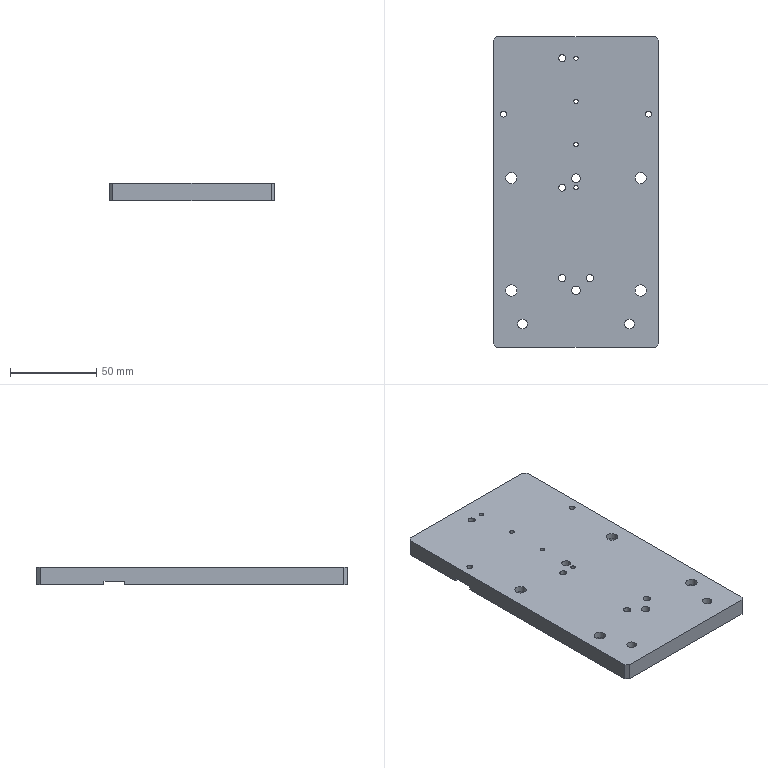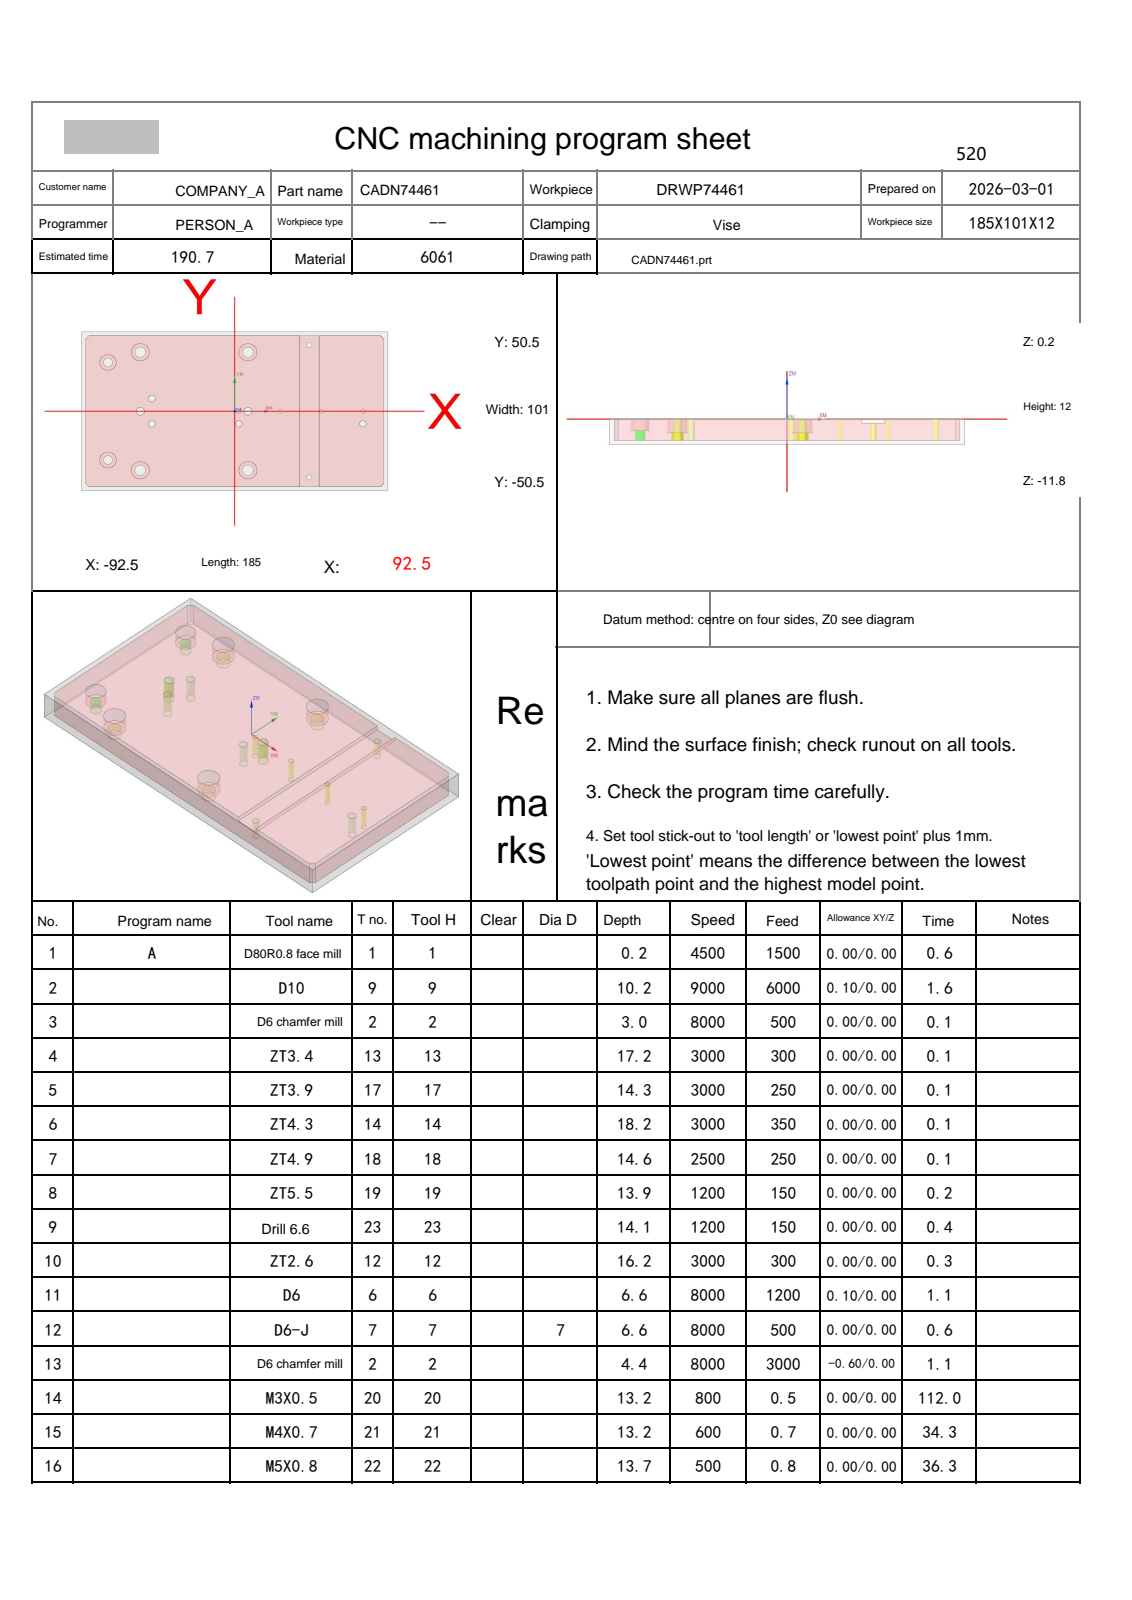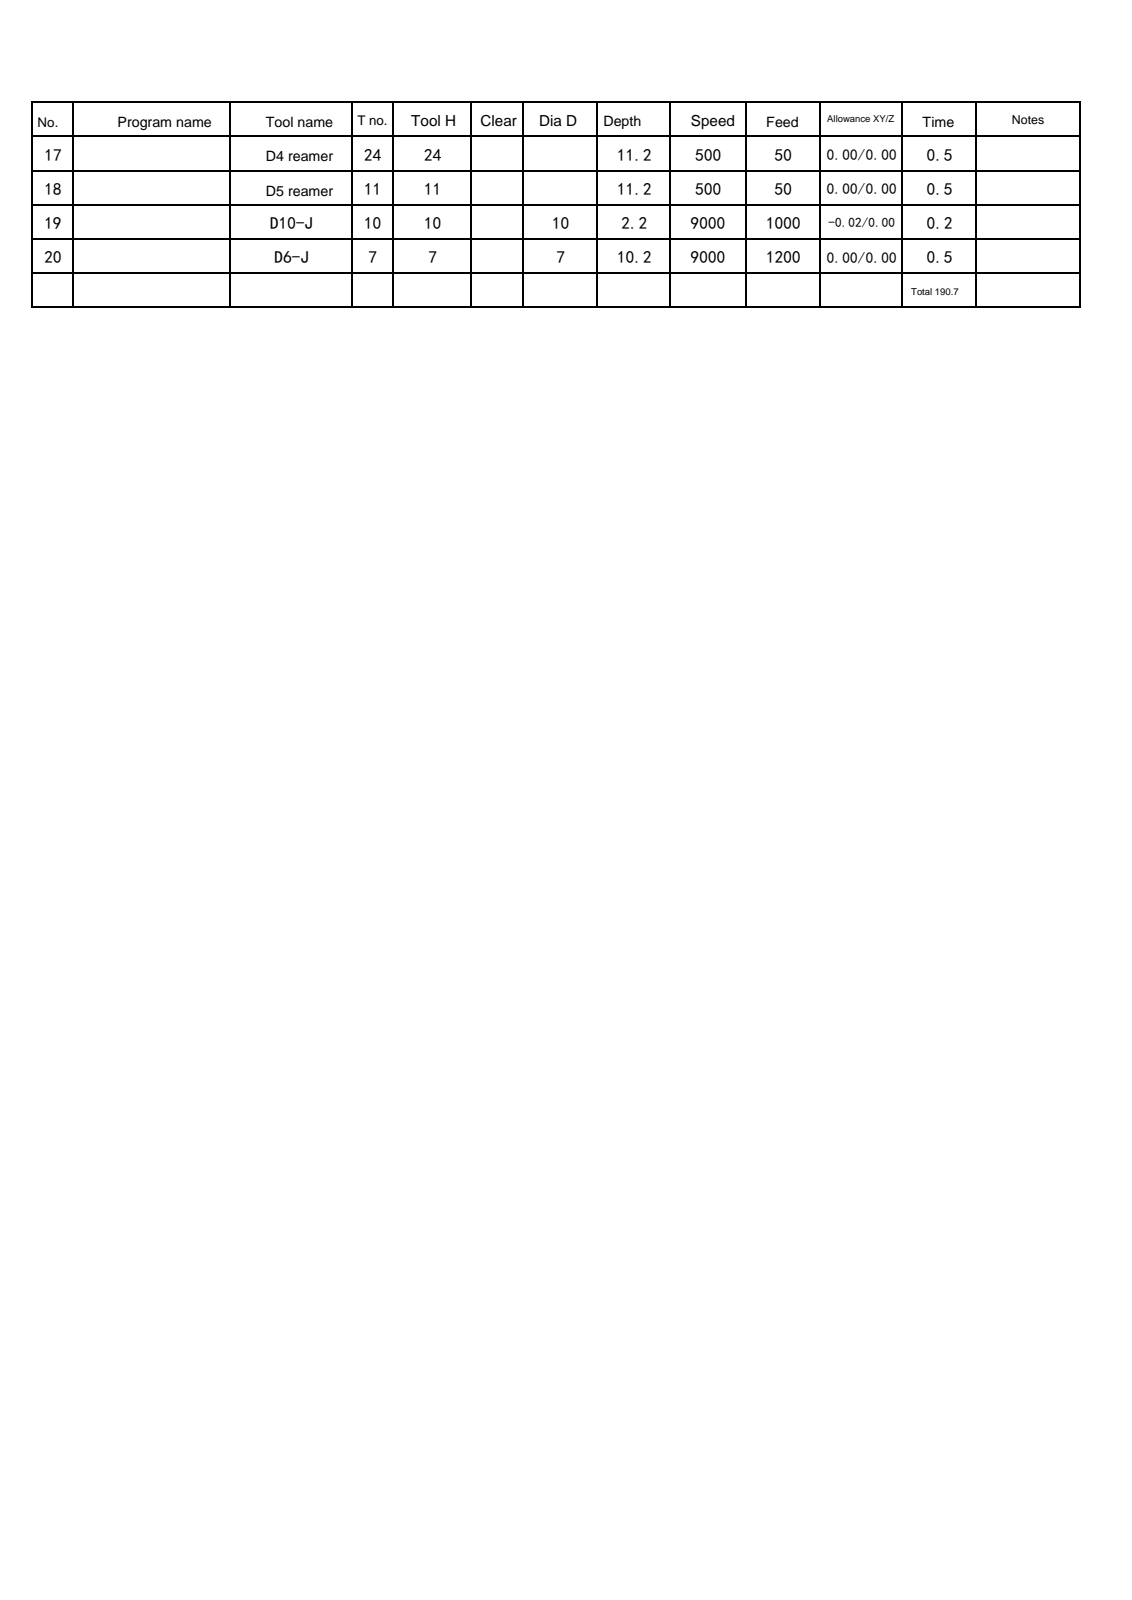NC program | NX | posted by the shop | part box 96 x 180 x 10 mm
Whole program:
%
O0001
(Machine time: 363.87 MIN)
(===Total Tool:18===)
(T1=D80R0.8 face mill D=80.  R=0.8  D-  H01 Z=0.    )
(T9=D10     D=10.  R=0.   D-  H09 Z=-10.  )
(T2=D6 chamfer mill   D=6.   R=0.   D-  H02 Z=-4.2  )
(T13=ZT3.4  D=3.4  DR_a=118 D-  H13 Z=-17.  )
(T17=ZT3.9  D=3.9  DR_a=120 D-  H17 Z=-14.13)
(T14=ZT4.3  D=4.3  DR_a=118 D-  H14 Z=-18.  )
(T18=ZT4.9  D=4.9  DR_a=120 D-  H18 Z=-14.41)
(T19=ZT5.5  D=5.5  DR_a=118 D-  H19 Z=-13.65)
(T23=drill 6.6  D=6.6  DR_a=120 D-  H23 Z=-13.91)
(T12=ZT2.6  D=2.6  DR_a=118 D-  H12 Z=-16.  )
(T6=D6      D=6.   R=0.   D-  H06 Z=-6.4  )
(T7=D6-J    D=6.   R=0.   D7  H07 Z=-10.  )
(T20=M3X0.5 D=2.5  DR_a=180 D-  H20 Z=-13.  )
(T21=M4X0.7 D=3.3  DR_a=180 D-  H21 Z=-13.  )
(T22=M5X0.8 D=4.2  DR_a=180 D-  H22 Z=-13.5 )
(T24=D4 reamer   D=4.   DR_a=180 D-  H24 Z=-11.  )
(T11=D5 reamer   D=5.   DR_a=180 D-  H11 Z=-11.  )
(T10=D10-J  D=10.  R=0.   D10 H10 Z=-2.   )
G80 G90 G17 G49 G40
G91 G28 Z0
M01
N1 T01 M06
(D80R0.8 face mill  D=80. R=0.8 H=01 ce=0.00 di=0.00)
G00 G90 G54 X-135. Y44. M03 S4500
G43 H01 Z50.
M08
Z2.
G01 Z0.0 F1500.
X-130.
X130.
Y0.0
X-130.
Y-44.
X130.
X135.
Z2.
G00 Z50.
G91 G28 Z0.0
M05
M09
G91 G28 Z0.0
M01
N2 T09 M06
(D10  D=10. R=0. H=09 ce=0.10 di=0.00)
G00 G90 G54 X0.0 Y-53.1 M03 S8000
G43 H09 Z50.
M08
Z.5
G01 X-88. Z.386 F6000.
G02 X-91.606 Y-51.606 Z.381 I0.0 J5.1
G01 X-93.606 Y-49.606 Z.377
G02 X-95.1 Y-46. Z.372 I3.606 J3.606
G01 Y46. Z.253
G02 X-93.606 Y49.606 Z.248 I5.1 J0.0
G01 X-91.606 Y51.606 Z.244
G02 X-88. Y53.1 Z.239 I3.606 J-3.606
G01 X88. Z.011
G02 X91.606 Y51.606 Z.006 I0.0 J-5.1
G01 X93.606 Y49.606 Z.002
G02 X95.1 Y46. Z-.003 I-3.606 J-3.606
G01 Y-46. Z-.122
G02 X93.606 Y-49.606 Z-.127 I-5.1 J0.0
G01 X91.606 Y-51.606 Z-.131
G02 X88. Y-53.1 Z-.136 I-3.606 J3.606
G01 X-88. Z-.364
G02 X-91.606 Y-51.606 Z-.369 I0.0 J5.1
G01 X-93.606 Y-49.606 Z-.373
G02 X-95.1 Y-46. Z-.378 I3.606 J3.606
G01 Y46. Z-.497
G02 X-93.606 Y49.606 Z-.502 I5.1 J0.0
G01 X-91.606 Y51.606 Z-.506
G02 X-88. Y53.1 Z-.511 I3.606 J-3.606
G01 X88. Z-.739
G02 X91.606 Y51.606 Z-.744 I0.0 J-5.1
G01 X93.606 Y49.606 Z-.748
G02 X95.1 Y46. Z-.753 I-3.606 J-3.606
G01 Y-46. Z-.872
G02 X93.606 Y-49.606 Z-.877 I-5.1 J0.0
G01 X91.606 Y-51.606 Z-.881
G02 X88. Y-53.1 Z-.886 I-3.606 J3.606
G01 X-88. Z-1.114
G02 X-91.606 Y-51.606 Z-1.119 I0.0 J5.1
G01 X-93.606 Y-49.606 Z-1.123
G02 X-95.1 Y-46. Z-1.128 I3.606 J3.606
G01 Y46. Z-1.247
G02 X-93.606 Y49.606 Z-1.252 I5.1 J0.0
G01 X-91.606 Y51.606 Z-1.256
G02 X-88. Y53.1 Z-1.261 I3.606 J-3.606
G01 X88. Z-1.489
G02 X91.606 Y51.606 Z-1.494 I0.0 J-5.1
G01 X93.606 Y49.606 Z-1.498
G02 X95.1 Y46. Z-1.503 I-3.606 J-3.606
G01 Y-46. Z-1.622
G02 X93.606 Y-49.606 Z-1.627 I-5.1 J0.0
G01 X91.606 Y-51.606 Z-1.631
G02 X88. Y-53.1 Z-1.636 I-3.606 J3.606
G01 X-88. Z-1.864
G02 X-91.606 Y-51.606 Z-1.869 I0.0 J5.1
G01 X-93.606 Y-49.606 Z-1.873
G02 X-95.1 Y-46. Z-1.878 I3.606 J3.606
G01 Y46. Z-1.997
G02 X-93.606 Y49.606 Z-2.002 I5.1 J0.0
G01 X-91.606 Y51.606 Z-2.006
G02 X-88. Y53.1 Z-2.011 I3.606 J-3.606
G01 X88. Z-2.239
G02 X91.606 Y51.606 Z-2.244 I0.0 J-5.1
G01 X93.606 Y49.606 Z-2.248
G02 X95.1 Y46. Z-2.253 I-3.606 J-3.606
G01 Y-46. Z-2.372
G02 X93.606 Y-49.606 Z-2.377 I-5.1 J0.0
G01 X91.606 Y-51.606 Z-2.381
G02 X88. Y-53.1 Z-2.386 I-3.606 J3.606
G01 X-88. Z-2.614
G02 X-91.606 Y-51.606 Z-2.619 I0.0 J5.1
G01 X-93.606 Y-49.606 Z-2.623
G02 X-95.1 Y-46. Z-2.628 I3.606 J3.606
G01 Y46. Z-2.747
G02 X-93.606 Y49.606 Z-2.752 I5.1 J0.0
G01 X-91.606 Y51.606 Z-2.756
G02 X-88. Y53.1 Z-2.761 I3.606 J-3.606
G01 X88. Z-2.989
G02 X91.606 Y51.606 Z-2.994 I0.0 J-5.1
G01 X93.606 Y49.606 Z-2.998
G02 X95.1 Y46. Z-3.003 I-3.606 J-3.606
G01 Y-46. Z-3.122
G02 X93.606 Y-49.606 Z-3.127 I-5.1 J0.0
G01 X91.606 Y-51.606 Z-3.131
G02 X88. Y-53.1 Z-3.136 I-3.606 J3.606
G01 X-88. Z-3.364
G02 X-91.606 Y-51.606 Z-3.369 I0.0 J5.1
G01 X-93.606 Y-49.606 Z-3.373
G02 X-95.1 Y-46. Z-3.378 I3.606 J3.606
G01 Y46. Z-3.497
G02 X-93.606 Y49.606 Z-3.502 I5.1 J0.0
G01 X-91.606 Y51.606 Z-3.506
G02 X-88. Y53.1 Z-3.511 I3.606 J-3.606
G01 X88. Z-3.739
G02 X91.606 Y51.606 Z-3.744 I0.0 J-5.1
G01 X93.606 Y49.606 Z-3.748
G02 X95.1 Y46. Z-3.753 I-3.606 J-3.606
G01 Y-46. Z-3.872
G02 X93.606 Y-49.606 Z-3.877 I-5.1 J0.0
G01 X91.606 Y-51.606 Z-3.881
G02 X88. Y-53.1 Z-3.886 I-3.606 J3.606
G01 X-88. Z-4.114
G02 X-91.606 Y-51.606 Z-4.119 I0.0 J5.1
G01 X-93.606 Y-49.606 Z-4.123
G02 X-95.1 Y-46. Z-4.128 I3.606 J3.606
G01 Y46. Z-4.247
G02 X-93.606 Y49.606 Z-4.252 I5.1 J0.0
G01 X-91.606 Y51.606 Z-4.256
G02 X-88. Y53.1 Z-4.261 I3.606 J-3.606
G01 X88. Z-4.489
G02 X91.606 Y51.606 Z-4.494 I0.0 J-5.1
G01 X93.606 Y49.606 Z-4.498
G02 X95.1 Y46. Z-4.503 I-3.606 J-3.606
G01 Y-46. Z-4.622
G02 X93.606 Y-49.606 Z-4.627 I-5.1 J0.0
G01 X91.606 Y-51.606 Z-4.631
G02 X88. Y-53.1 Z-4.636 I-3.606 J3.606
G01 X-88. Z-4.864
G02 X-91.606 Y-51.606 Z-4.869 I0.0 J5.1
G01 X-93.606 Y-49.606 Z-4.873
G02 X-95.1 Y-46. Z-4.878 I3.606 J3.606
G01 Y46. Z-4.997
G02 X-93.606 Y49.606 Z-5.002 I5.1 J0.0
G01 X-91.606 Y51.606 Z-5.006
G02 X-88. Y53.1 Z-5.011 I3.606 J-3.606
G01 X88. Z-5.239
G02 X91.606 Y51.606 Z-5.244 I0.0 J-5.1
G01 X93.606 Y49.606 Z-5.248
G02 X95.1 Y46. Z-5.253 I-3.606 J-3.606
G01 Y-46. Z-5.372
G02 X93.606 Y-49.606 Z-5.377 I-5.1 J0.0
G01 X91.606 Y-51.606 Z-5.381
G02 X88. Y-53.1 Z-5.386 I-3.606 J3.606
G01 X-88. Z-5.614
G02 X-91.606 Y-51.606 Z-5.619 I0.0 J5.1
G01 X-93.606 Y-49.606 Z-5.623
G02 X-95.1 Y-46. Z-5.628 I3.606 J3.606
G01 Y46. Z-5.747
G02 X-93.606 Y49.606 Z-5.752 I5.1 J0.0
G01 X-91.606 Y51.606 Z-5.756
G02 X-88. Y53.1 Z-5.761 I3.606 J-3.606
G01 X88. Z-5.989
G02 X91.606 Y51.606 Z-5.994 I0.0 J-5.1
G01 X93.606 Y49.606 Z-5.998
G02 X95.1 Y46. Z-6.003 I-3.606 J-3.606
G01 Y-46. Z-6.122
G02 X93.606 Y-49.606 Z-6.127 I-5.1 J0.0
G01 X91.606 Y-51.606 Z-6.131
G02 X88. Y-53.1 Z-6.136 I-3.606 J3.606
G01 X-88. Z-6.364
G02 X-91.606 Y-51.606 Z-6.369 I0.0 J5.1
G01 X-93.606 Y-49.606 Z-6.373
G02 X-95.1 Y-46. Z-6.378 I3.606 J3.606
G01 Y46. Z-6.497
G02 X-93.606 Y49.606 Z-6.502 I5.1 J0.0
G01 X-91.606 Y51.606 Z-6.506
G02 X-88. Y53.1 Z-6.511 I3.606 J-3.606
G01 X88. Z-6.739
G02 X91.606 Y51.606 Z-6.744 I0.0 J-5.1
G01 X93.606 Y49.606 Z-6.748
G02 X95.1 Y46. Z-6.753 I-3.606 J-3.606
G01 Y-46. Z-6.872
G02 X93.606 Y-49.606 Z-6.877 I-5.1 J0.0
G01 X91.606 Y-51.606 Z-6.881
G02 X88. Y-53.1 Z-6.886 I-3.606 J3.606
G01 X-88. Z-7.114
G02 X-91.606 Y-51.606 Z-7.119 I0.0 J5.1
G01 X-93.606 Y-49.606 Z-7.123
G02 X-95.1 Y-46. Z-7.128 I3.606 J3.606
G01 Y46. Z-7.247
G02 X-93.606 Y49.606 Z-7.252 I5.1 J0.0
G01 X-91.606 Y51.606 Z-7.256
G02 X-88. Y53.1 Z-7.261 I3.606 J-3.606
G01 X88. Z-7.489
G02 X91.606 Y51.606 Z-7.494 I0.0 J-5.1
G01 X93.606 Y49.606 Z-7.498
G02 X95.1 Y46. Z-7.503 I-3.606 J-3.606
G01 Y-46. Z-7.622
G02 X93.606 Y-49.606 Z-7.627 I-5.1 J0.0
G01 X91.606 Y-51.606 Z-7.631
G02 X88. Y-53.1 Z-7.636 I-3.606 J3.606
G01 X-88. Z-7.864
G02 X-91.606 Y-51.606 Z-7.869 I0.0 J5.1
G01 X-93.606 Y-49.606 Z-7.873
G02 X-95.1 Y-46. Z-7.878 I3.606 J3.606
G01 Y46. Z-7.997
G02 X-93.606 Y49.606 Z-8.002 I5.1 J0.0
G01 X-91.606 Y51.606 Z-8.006
G02 X-88. Y53.1 Z-8.011 I3.606 J-3.606
G01 X88. Z-8.239
G02 X91.606 Y51.606 Z-8.244 I0.0 J-5.1
G01 X93.606 Y49.606 Z-8.248
G02 X95.1 Y46. Z-8.253 I-3.606 J-3.606
G01 Y-46. Z-8.372
G02 X93.606 Y-49.606 Z-8.377 I-5.1 J0.0
G01 X91.606 Y-51.606 Z-8.381
G02 X88. Y-53.1 Z-8.386 I-3.606 J3.606
G01 X-88. Z-8.614
G02 X-91.606 Y-51.606 Z-8.619 I0.0 J5.1
G01 X-93.606 Y-49.606 Z-8.623
G02 X-95.1 Y-46. Z-8.628 I3.606 J3.606
G01 Y46. Z-8.747
G02 X-93.606 Y49.606 Z-8.752 I5.1 J0.0
G01 X-91.606 Y51.606 Z-8.756
G02 X-88. Y53.1 Z-8.761 I3.606 J-3.606
G01 X88. Z-8.989
G02 X91.606 Y51.606 Z-8.994 I0.0 J-5.1
G01 X93.606 Y49.606 Z-8.998
G02 X95.1 Y46. Z-9.003 I-3.606 J-3.606
G01 Y-46. Z-9.122
G02 X93.606 Y-49.606 Z-9.127 I-5.1 J0.0
G01 X91.606 Y-51.606 Z-9.131
G02 X88. Y-53.1 Z-9.136 I-3.606 J3.606
G01 X-88. Z-9.364
G02 X-91.606 Y-51.606 Z-9.369 I0.0 J5.1
G01 X-93.606 Y-49.606 Z-9.373
G02 X-95.1 Y-46. Z-9.378 I3.606 J3.606
G01 Y46. Z-9.497
G02 X-93.606 Y49.606 Z-9.502 I5.1 J0.0
G01 X-91.606 Y51.606 Z-9.506
G02 X-88. Y53.1 Z-9.511 I3.606 J-3.606
G01 X88. Z-9.739
G02 X91.606 Y51.606 Z-9.744 I0.0 J-5.1
G01 X93.606 Y49.606 Z-9.748
G02 X95.1 Y46. Z-9.753 I-3.606 J-3.606
G01 Y-46. Z-9.872
G02 X93.606 Y-49.606 Z-9.877 I-5.1 J0.0
G01 X91.606 Y-51.606 Z-9.881
G02 X88. Y-53.1 Z-9.886 I-3.606 J3.606
G01 X0.0 Z-10.
X-88.
G02 X-91.606 Y-51.606 I0.0 J5.1
G01 X-93.606 Y-49.606
G02 X-95.1 Y-46. I3.606 J3.606
G01 Y46.
G02 X-93.606 Y49.606 I5.1 J0.0
G01 X-91.606 Y51.606
G02 X-88. Y53.1 I3.606 J-3.606
G01 X88.
G02 X91.606 Y51.606 I0.0 J-5.1
G01 X93.606 Y49.606
G02 X95.1 Y46. I-3.606 J-3.606
G01 Y-46.
G02 X93.606 Y-49.606 I-5.1 J0.0
G01 X91.606 Y-51.606
G02 X88. Y-53.1 I-3.606 J3.606
G01 X0.0
X-.5
Z-9.
G00 Z50.
G00 G90 X45. Y56.1 M03 S9000
Z50.
Z.025
G01 Z-.475 F6000.
Y49.
X44.1
Y-49.
X45.9
Y49.
X45.
X44.5
Z.025
G00 Z50.
X45. Y56.1
Z-.45
G01 Z-.95
Y49.
X44.1
Y-49.
X45.9
Y49.
X45.
X44.5
Z-.45
G00 Z.025
X45. Y56.1
Z-.925
G01 Z-1.425
Y49.
X44.1
Y-49.
X45.9
Y49.
X45.
X44.5
Z-.925
G00 Z-.45
X45. Y56.1
Z-1.4
G01 Z-1.9
Y49.
X44.1
Y-49.
X45.9
Y49.
X45.
X44.5
Z-1.4
G00 Z50.
G91 G28 Z0.0
M05
M09
G91 G28 Z0.0
M01
N3 T02 M06
(D6 chamfer mill  D=6. R=0. H=02 ce=0.00 di=0.10)
G00 G90 G54 X-76.5 Y31. M03 S8000
G43 H02 Z50.
M08
G98 G81 X-76.5 Y31. Z-.8 R1. F500.
X-57. Y37.5
X-50. Y8.
X-57. Y0.0
X-50. Y-8.
X-76.5 Y-31.
X-57. Y-37.5
X8.
X45. Y-42. Z-2.8 R-1.
X77.5 Y-8. Z-.8 R1.
Y0.0
X52.5
X27.5
X8.
X2.5 Y-8.
Y0.0
X8. Y37.5
X45. Y42. Z-2.8 R-1.
G80
G00 Z50.
G91 G28 Z0.0
M05
M09
G91 G28 Z0.0
M01
N4 T13 M06
(ZT3.4 D=3.4 DR_a=118 H=13)
G00 G90 G54 X45. Y-42. M03 S3000
G43 H13 Z50.
M08
G98 G83 X45. Y-42. Z-17. R-1. F300. Q2.
Y42.
G80
G00 Z50.
G91 G28 Z0.0
M05
M09
G91 G28 Z0.0
M01
N5 T17 M06
(ZT3.9 D=3.9 DR_a=120 H=17)
G00 G90 G54 X2.5 Y-8. M03 S3000
G43 H17 Z50.
M08
G98 G83 X2.5 Y-8. Z-14.126 R1. F250. Q2.
X77.5
G80
G00 Z50.
G91 G28 Z0.0
M05
M09
G91 G28 Z0.0
M01
N6 T14 M06
(ZT4.3 D=4.3 DR_a=118 H=14)
G00 G90 G54 X-50. Y8. M03 S3000
G43 H14 Z50.
M08
G98 G83 X-50. Y8. Z-18. R1. F350. Q3.
Y-8.
G80
G00 Z50.
G91 G28 Z0.0
M05
M09
G91 G28 Z0.0
M01
N7 T18 M06
(ZT4.9 D=4.9 DR_a=120 H=18)
G00 G90 G54 X8. Y0.0 M03 S2500
G43 H18 Z50.
M08
G98 G83 X8. Y0.0 Z-14.415 R1. F250. Q2.
X-57.
G80
G00 Z50.
G91 G28 Z0.0
M05
M09
G91 G28 Z0.0
M01
N8 T19 M06
(ZT5.5 D=5.5 DR_a=118 H=19)
G00 G90 G54 X-76.5 Y31. M03 S1200
G43 H19 Z50.
M08
G98 G83 X-76.5 Y31. Z-13.652 R1. F150. Q2.
Y-31.
G80
G00 Z50.
G91 G28 Z0.0
M05
M09
G91 G28 Z0.0
M01
N9 T23 M06
(drill 6.6 D=6.6 DR_a=120 H=23)
G00 G90 G54 X-57. Y-37.5 M03 S1200
G43 H23 Z50.
M08
G98 G83 X-57. Y-37.5 Z-13.905 R1. F150. Q2.
X8.
Y37.5
X-57.
G80
G00 Z50.
G91 G28 Z0.0
M05
M09
G91 G28 Z0.0
M01
N10 T12 M06
(ZT2.6 D=2.6 DR_a=118 H=12)
G00 G90 G54 X2.5 Y0.0 M03 S3000
G43 H12 Z50.
M08
G98 G83 X2.5 Y0.0 Z-16. R1. F300. Q2.
X27.5
X52.5
X77.5
G80
G00 Z50.
G91 G28 Z0.0
M05
M09
G91 G28 Z0.0
M01
N11 T06 M06
(D6  D=6. R=0. H=06 ce=0.10 di=0.00)
G00 G90 G54 X-76.5 Y31. M03 S8000
G43 H06 Z50.
M08
Z.5
G03 X-75.55 Y31.95 I0.0 J.95 F1200.
X-76.5 Y32.9 I-.95 J0.0
X-76.5 Y32.9 Z0.0 I0.0 J-1.9
X-76.5 Y32.9 Z-.5 I0.0 J-1.9
X-76.5 Y32.9 Z-1. I0.0 J-1.9
X-76.5 Y32.9 Z-1.5 I0.0 J-1.9
X-76.5 Y32.9 Z-2. I0.0 J-1.9
X-76.5 Y32.9 Z-2.5 I0.0 J-1.9
X-76.5 Y32.9 Z-3. I0.0 J-1.9
X-76.5 Y32.9 Z-3.5 I0.0 J-1.9
X-76.5 Y32.9 Z-4. I0.0 J-1.9
X-76.5 Y32.9 Z-4.5 I0.0 J-1.9
X-76.5 Y32.9 Z-5. I0.0 J-1.9
X-74.693 Y31.587 Z-5.4 I0.0 J-1.9
X-76.5 Y32.9 I-1.807 J-.587
X-78.4 Y31. I0.0 J-1.9
X-76.5 Y29.1 I1.9 J0.0
X-74.6 Y31. I0.0 J1.9
X-74.693 Y31.587 I-1.9 J0.0
X-75.596 Y32.244 I-.904 J-.294
X-76.546 Y31.294 I0.0 J-.95
X-76.5 Y31. I.95 J0.0
G00 Z50.
Y-31.
Z.5
G03 X-75.55 Y-30.05 I0.0 J.95
X-76.5 Y-29.1 I-.95 J0.0
X-76.5 Y-29.1 Z0.0 I0.0 J-1.9
X-76.5 Y-29.1 Z-.5 I0.0 J-1.9
X-76.5 Y-29.1 Z-1. I0.0 J-1.9
X-76.5 Y-29.1 Z-1.5 I0.0 J-1.9
X-76.5 Y-29.1 Z-2. I0.0 J-1.9
X-76.5 Y-29.1 Z-2.5 I0.0 J-1.9
X-76.5 Y-29.1 Z-3. I0.0 J-1.9
X-76.5 Y-29.1 Z-3.5 I0.0 J-1.9
X-76.5 Y-29.1 Z-4. I0.0 J-1.9
X-76.5 Y-29.1 Z-4.5 I0.0 J-1.9
X-76.5 Y-29.1 Z-5. I0.0 J-1.9
X-74.693 Y-30.413 Z-5.4 I0.0 J-1.9
X-76.5 Y-29.1 I-1.807 J-.587
X-78.4 Y-31. I0.0 J-1.9
X-76.5 Y-32.9 I1.9 J0.0
X-74.6 Y-31. I0.0 J1.9
X-74.693 Y-30.413 I-1.9 J0.0
X-75.596 Y-29.756 I-.904 J-.294
X-76.546 Y-30.706 I0.0 J-.95
X-76.5 Y-31. I.95 J0.0
G00 Z50.
G00 G90 X-57. Y-37.5 M03 S8000
Z50.
Z.5
G03 X-55.8 Y-36.3 I0.0 J1.2 F1200.
X-57. Y-35.1 I-1.2 J0.0
X-57. Y-35.1 Z0.0 I0.0 J-2.4
X-57. Y-35.1 Z-.5 I0.0 J-2.4
X-57. Y-35.1 Z-1. I0.0 J-2.4
X-57. Y-35.1 Z-1.5 I0.0 J-2.4
X-57. Y-35.1 Z-2. I0.0 J-2.4
X-57. Y-35.1 Z-2.5 I0.0 J-2.4
X-57. Y-35.1 Z-3. I0.0 J-2.4
X-57. Y-35.1 Z-3.5 I0.0 J-2.4
X-57. Y-35.1 Z-4. I0.0 J-2.4
X-57. Y-35.1 Z-4.5 I0.0 J-2.4
X-57. Y-35.1 Z-5. I0.0 J-2.4
X-57. Y-35.1 Z-5.5 I0.0 J-2.4
X-57. Y-35.1 Z-6. I0.0 J-2.4
X-54.717 Y-36.758 Z-6.4 I0.0 J-2.4
X-57. Y-35.1 I-2.283 J-.742
X-59.4 Y-37.5 I0.0 J-2.4
X-57. Y-39.9 I2.4 J0.0
X-54.6 Y-37.5 I0.0 J2.4
X-54.717 Y-36.758 I-2.4 J0.0
X-55.859 Y-35.929 I-1.141 J-.371
X-57.059 Y-37.129 I0.0 J-1.2
X-57. Y-37.5 I1.2 J0.0
G00 Z50.
X8.
Z.5
G03 X9.2 Y-36.3 I0.0 J1.2
X8. Y-35.1 I-1.2 J0.0
X8. Y-35.1 Z0.0 I0.0 J-2.4
X8. Y-35.1 Z-.5 I0.0 J-2.4
X8. Y-35.1 Z-1. I0.0 J-2.4
X8. Y-35.1 Z-1.5 I0.0 J-2.4
X8. Y-35.1 Z-2. I0.0 J-2.4
X8. Y-35.1 Z-2.5 I0.0 J-2.4
X8. Y-35.1 Z-3. I0.0 J-2.4
X8. Y-35.1 Z-3.5 I0.0 J-2.4
X8. Y-35.1 Z-4. I0.0 J-2.4
X8. Y-35.1 Z-4.5 I0.0 J-2.4
X8. Y-35.1 Z-5. I0.0 J-2.4
X8. Y-35.1 Z-5.5 I0.0 J-2.4
X8. Y-35.1 Z-6. I0.0 J-2.4
X10.283 Y-36.758 Z-6.4 I0.0 J-2.4
X8. Y-35.1 I-2.283 J-.742
X5.6 Y-37.5 I0.0 J-2.4
X8. Y-39.9 I2.4 J0.0
X10.4 Y-37.5 I0.0 J2.4
X10.283 Y-36.758 I-2.4 J0.0
X9.141 Y-35.929 I-1.141 J-.371
X7.941 Y-37.129 I0.0 J-1.2
X8. Y-37.5 I1.2 J0.0
G00 Z50.
Y37.5
Z.5
G03 X9.2 Y38.7 I0.0 J1.2
X8. Y39.9 I-1.2 J0.0
X8. Y39.9 Z0.0 I0.0 J-2.4
X8. Y39.9 Z-.5 I0.0 J-2.4
X8. Y39.9 Z-1. I0.0 J-2.4
X8. Y39.9 Z-1.5 I0.0 J-2.4
X8. Y39.9 Z-2. I0.0 J-2.4
X8. Y39.9 Z-2.5 I0.0 J-2.4
X8. Y39.9 Z-3. I0.0 J-2.4
X8. Y39.9 Z-3.5 I0.0 J-2.4
X8. Y39.9 Z-4. I0.0 J-2.4
X8. Y39.9 Z-4.5 I0.0 J-2.4
X8. Y39.9 Z-5. I0.0 J-2.4
X8. Y39.9 Z-5.5 I0.0 J-2.4
X8. Y39.9 Z-6. I0.0 J-2.4
X10.283 Y38.242 Z-6.4 I0.0 J-2.4
X8. Y39.9 I-2.283 J-.742
X5.6 Y37.5 I0.0 J-2.4
X8. Y35.1 I2.4 J0.0
X10.4 Y37.5 I0.0 J2.4
X10.283 Y38.242 I-2.4 J0.0
X9.141 Y39.071 I-1.141 J-.371
X7.941 Y37.871 I0.0 J-1.2
X8. Y37.5 I1.2 J0.0
G00 Z50.
X-57.
Z.5
G03 X-55.8 Y38.7 I0.0 J1.2
X-57. Y39.9 I-1.2 J0.0
X-57. Y39.9 Z0.0 I0.0 J-2.4
X-57. Y39.9 Z-.5 I0.0 J-2.4
X-57. Y39.9 Z-1. I0.0 J-2.4
X-57. Y39.9 Z-1.5 I0.0 J-2.4
X-57. Y39.9 Z-2. I0.0 J-2.4
X-57. Y39.9 Z-2.5 I0.0 J-2.4
X-57. Y39.9 Z-3. I0.0 J-2.4
X-57. Y39.9 Z-3.5 I0.0 J-2.4
X-57. Y39.9 Z-4. I0.0 J-2.4
X-57. Y39.9 Z-4.5 I0.0 J-2.4
X-57. Y39.9 Z-5. I0.0 J-2.4
X-57. Y39.9 Z-5.5 I0.0 J-2.4
X-57. Y39.9 Z-6. I0.0 J-2.4
X-54.717 Y38.242 Z-6.4 I0.0 J-2.4
X-57. Y39.9 I-2.283 J-.742
X-59.4 Y37.5 I0.0 J-2.4
X-57. Y35.1 I2.4 J0.0
X-54.6 Y37.5 I0.0 J2.4
X-54.717 Y38.242 I-2.4 J0.0
X-55.859 Y39.071 I-1.141 J-.371
X-57.059 Y37.871 I0.0 J-1.2
X-57. Y37.5 I1.2 J0.0
G00 Z50.
G91 G28 Z0.0
M05
M09
G91 G28 Z0.0
M01
N12 T07 M06
(D6-J  D=6. R=0. H=07 ce=0.00 di=0.00)
G00 G90 G54 X-76.5 Y31. M03 S8000
G43 H07 Z50.
M08
Z0.0
G41 D07
G01 X-76.304 Y31.04 F500.
G03 X-75.51 Y32.01 I-.196 J.97
X-76.5 Y33. I-.99 J0.0
X-76.5 Y33. Z-5. I0.0 J-2.
X-77.464 Y32.753 Z-5.4 I0.0 J-2.
X-78.5 Y31. I.964 J-1.753
X-76.5 Y29. I2. J0.0
X-74.5 Y31. I0.0 J2.
X-76.5 Y33. I-2. J0.0
X-77.464 Y32.753 I0.0 J-2.
X-77.977 Y31.885 I.477 J-.868
X-76.987 Y30.895 I.99 J0.0
X-76.691 Y30.94 I0.0 J.99
G01 G40 X-76.5 Y31.
G00 Z50.
Y-31.
Z0.0
G41 D07
G01 X-76.304 Y-30.96
G03 X-75.51 Y-29.99 I-.196 J.97
X-76.5 Y-29. I-.99 J0.0
X-76.5 Y-29. Z-5. I0.0 J-2.
X-77.464 Y-29.247 Z-5.4 I0.0 J-2.
X-78.5 Y-31. I.964 J-1.753
X-76.5 Y-33. I2. J0.0
X-74.5 Y-31. I0.0 J2.
X-76.5 Y-29. I-2. J0.0
X-77.464 Y-29.247 I0.0 J-2.
X-77.977 Y-30.115 I.477 J-.868
X-76.987 Y-31.105 I.99 J0.0
X-76.691 Y-31.06 I0.0 J.99
G01 G40 X-76.5 Y-31.
G00 Z50.
G00 G90 X-57. Y-37.5 M03 S8000
Z50.
Z0.0
G41 D07
G01 X-56.803 Y-37.468 F500.
G03 X-55.758 Y-36.242 I-.197 J1.226
X-57. Y-35. I-1.242 J0.0
X-57. Y-35. Z-5. I0.0 J-2.5
X-59.456 Y-37.968 Z-6.4 I0.0 J-2.5
X-57. Y-40. I2.456 J.468
X-54.5 Y-37.5 I0.0 J2.5
X-57. Y-35. I-2.5 J0.0
X-59.5 Y-37.5 I0.0 J-2.5
X-59.456 Y-37.968 I2.5 J0.0
X-58.236 Y-38.978 I1.22 J.233
X-56.994 Y-37.736 I0.0 J1.242
G01 Y-37.7
G40 X-57. Y-37.5
G00 Z50.
X8.
Z0.0
G41 D07
G01 X8.197 Y-37.468
G03 X9.242 Y-36.242 I-.197 J1.226
X8. Y-35. I-1.242 J0.0
X8. Y-35. Z-5. I0.0 J-2.5
X5.544 Y-37.968 Z-6.4 I0.0 J-2.5
X8. Y-40. I2.456 J.468
X10.5 Y-37.5 I0.0 J2.5
X8. Y-35. I-2.5 J0.0
X5.5 Y-37.5 I0.0 J-2.5
X5.544 Y-37.968 I2.5 J0.0
X6.764 Y-38.978 I1.22 J.233
X8.006 Y-37.736 I0.0 J1.242
G01 Y-37.7
G40 X8. Y-37.5
G00 Z50.
Y37.5
Z0.0
G41 D07
G01 X8.197 Y37.532
G03 X9.242 Y38.758 I-.197 J1.226
X8. Y40. I-1.242 J0.0
X8. Y40. Z-5. I0.0 J-2.5
X5.544 Y37.032 Z-6.4 I0.0 J-2.5
X8. Y35. I2.456 J.468
X10.5 Y37.5 I0.0 J2.5
X8. Y40. I-2.5 J0.0
X5.5 Y37.5 I0.0 J-2.5
X5.544 Y37.032 I2.5 J0.0
X6.764 Y36.022 I1.22 J.233
X8.006 Y37.264 I0.0 J1.242
G01 Y37.3
G40 X8. Y37.5
G00 Z50.
X-57.
Z0.0
G41 D07
G01 X-56.803 Y37.532
G03 X-55.758 Y38.758 I-.197 J1.226
X-57. Y40. I-1.242 J0.0
X-57. Y40. Z-5. I0.0 J-2.5
X-59.456 Y37.032 Z-6.4 I0.0 J-2.5
X-57. Y35. I2.456 J.468
X-54.5 Y37.5 I0.0 J2.5
X-57. Y40. I-2.5 J0.0
X-59.5 Y37.5 I0.0 J-2.5
X-59.456 Y37.032 I2.5 J0.0
X-58.236 Y36.022 I1.22 J.233
X-56.994 Y37.264 I0.0 J1.242
G01 Y37.3
G40 X-57. Y37.5
G00 Z50.
G91 G28 Z0.0
M05
M09
G91 G28 Z0.0
M01
N13 T02 M06
(D6 chamfer mill  D=6. R=0. H=02 ce=0.00 di=0.00)
G00 G90 G54 X-24.25 Y-50.128 M03 S8000
G43 H02 Z50.
M08
Z2.099
G01 Z-1.5 F3000.
G03 X-24.17 Y-49.828 I-.52 J.3
X-24.47 Y-49.308 I-.6 J0.0
G01 X-24.5 Y-49.3
X-88.
X-88.254 Y-49.275
X-88.497 Y-49.201
X-88.722 Y-49.081
X-88.919 Y-48.919
X-90.919 Y-46.919
X-91.081 Y-46.722
X-91.201 Y-46.497
X-91.275 Y-46.254
X-91.3 Y-46.
Y46.
X-91.275 Y46.254
X-91.201 Y46.497
X-91.081 Y46.722
X-90.919 Y46.919
X-88.919 Y48.919
X-88.722 Y49.081
X-88.497 Y49.201
X-88.254 Y49.275
X-88. Y49.3
X39.
G02 X40.3 Y48. I0.0 J-1.3
G01 Y-48.
G02 X39. Y-49.3 I-1.3 J0.0
G01 X-24.5
X-24.53 Y-49.308
G03 X-24.83 Y-49.828 I.3 J-.52
X-24.75 Y-50.128 I.6 J0.0
G01 Z2.099
G00 Z50.
X48.872 Y-.25
Z2.099
G01 Z-1.5
G03 X49.172 Y-.33 I.3 J.52
X49.692 Y-.03 I0.0 J.6
G01 X49.7 Y0.0
Y48.
G02 X51. Y49.3 I1.3 J0.0
G01 X88.
X88.254 Y49.275
X88.497 Y49.201
X88.722 Y49.081
X88.919 Y48.919
X90.919 Y46.919
X91.081 Y46.722
X91.201 Y46.497
X91.275 Y46.254
X91.3 Y46.
Y-46.
X91.275 Y-46.254
X91.201 Y-46.497
X91.081 Y-46.722
X90.919 Y-46.919
X88.919 Y-48.919
X88.722 Y-49.081
X88.497 Y-49.201
X88.254 Y-49.275
X88. Y-49.3
X51.
G02 X49.7 Y-48. I0.0 J1.3
G01 Y0.0
X49.692 Y.03
G03 X49.172 Y.33 I-.52 J-.3
X48.872 Y.25 I0.0 J-.6
G01 Z2.099
G00 Z50.
X47.968 Y-50.128
Z1.755
G01 Z-3.499
G03 X48.049 Y-49.828 I-.52 J.3
X47.749 Y-49.308 I-.6 J0.0
G01 X47.719 Y-49.3
X42.281
X42.251 Y-49.308
G03 X41.951 Y-49.828 I.3 J-.52
X42.032 Y-50.128 I.6 J0.0
G01 Z1.755
G00 Z50.
Y50.128
Z1.755
G01 Z-3.499
G03 X41.951 Y49.828 I.52 J-.3
X42.251 Y49.308 I.6 J0.0
G01 X42.281 Y49.3
X47.719
X47.749 Y49.308
G03 X48.049 Y49.828 I-.3 J.52
X47.968 Y50.128 I-.6 J0.0
G01 Z1.755
G00 Z50.
G00 G90 X2.5 Y0.0 M03 S8000
Z50.
G98 G81 X2.5 Y0.0 Z-1.75 R3. F500.
X27.5
X52.5
X77.5
G80
G00 Z50.
G00 G90 X45. Y-42. M03 S8000
Z50.
G98 G81 X45. Y-42. Z-4.2 R1. F500.
Y42.
G80
G00 Z50.
G00 G90 X2.5 Y-8. M03 S8000
Z50.
G98 G81 X2.5 Y-8. Z-2.3 R3. F500.
X77.5
G80
G00 Z50.
G00 G90 X-49.306 Y8.093 M03 S8000
Z50.
Z-.5
G01 Z-1. F500.
X-48.5 Y8.2
G03 X-50. Y9.7 I-1.5 J0.0
X-51.7 Y8. I0.0 J-1.7
X-50. Y6.3 I1.7 J0.0
X-48.3 Y8. I0.0 J1.7
X-50. Y9.7 I-1.7 J0.0
X-51.5 Y8.2 I0.0 J-1.5
G01 X-50.694 Y8.093
Z-.5
G00 Z50.
X-49.306 Y-7.907
Z-.5
G01 Z-1.
X-48.5 Y-7.8
G03 X-50. Y-6.3 I-1.5 J0.0
X-51.7 Y-8. I0.0 J-1.7
X-50. Y-9.7 I1.7 J0.0
X-48.3 Y-8. I0.0 J1.7
X-50. Y-6.3 I-1.7 J0.0
X-51.5 Y-7.8 I0.0 J-1.5
G01 X-50.694 Y-7.907
Z-.5
G00 Z50.
G00 G90 X7.216 Y-.157 M03 S8000
Z50.
Z-.5
G01 Z-1. F500.
X6.5 Y-.3
G03 X8. Y-1.8 I1.5 J0.0
X9.8 Y0.0 I0.0 J1.8
X8. Y1.8 I-1.8 J0.0
X6.2 Y0.0 I0.0 J-1.8
X8. Y-1.8 I1.8 J0.0
X9.5 Y-.3 I0.0 J1.5
G01 X8.784 Y-.157
Z-.5
G00 Z50.
X-57.784
Z-.5
G01 Z-1.
X-58.5 Y-.3
G03 X-57. Y-1.8 I1.5 J0.0
X-55.2 Y0.0 I0.0 J1.8
X-57. Y1.8 I-1.8 J0.0
X-58.8 Y0.0 I0.0 J-1.8
X-57. Y-1.8 I1.8 J0.0
X-55.5 Y-.3 I0.0 J1.5
G01 X-56.216 Y-.157
Z-.5
G00 Z50.
G00 G90 X-79.886 Y33.654 M03 S8000
Z50.
Z2.5
G01 X-79.894 Y33.645 Z2.495 F800.
X-80.144 Y33.289 Z2.337
X-80.304 Y33.011 Z2.22
X-80.488 Y32.617 Z2.062
X-80.63 Y32.207 Z1.904
X-80.731 Y31.784 Z1.746
X-80.788 Y31.354 Z1.588
X-80.802 Y30.92 Z1.43
X-80.772 Y30.486 Z1.272
X-80.699 Y30.058 Z1.114
X-80.582 Y29.64 Z.956
X-80.424 Y29.235 Z.797
X-80.227 Y28.849 Z.639
X-79.991 Y28.484 Z.481
X-79.719 Y28.145 Z.323
X-79.415 Y27.835 Z.165
X-79.081 Y27.557 Z.007
X-78.721 Y27.314 Z-.151
X-78.338 Y27.109 Z-.309
X-77.936 Y26.944 Z-.467
X-77.52 Y26.82 Z-.625
X-77.093 Y26.738 Z-.783
X-76.661 Y26.7 Z-.942
X-76.5 Z-1.
G03 X-72.2 Y31. I0.0 J4.3
X-76.5 Y35.3 I-4.3 J0.0
X-80.8 Y31. I0.0 J-4.3
X-76.5 Y26.7 I4.3 J0.0
X-76.001 Y26.729 I0.0 J4.3
G01 Z1.5
G00 Z50.
X-79.886 Y-28.346
Z2.5
G01 X-79.894 Y-28.355 Z2.495
X-80.144 Y-28.711 Z2.337
X-80.304 Y-28.989 Z2.22
X-80.488 Y-29.383 Z2.062
X-80.63 Y-29.793 Z1.904
X-80.731 Y-30.216 Z1.746
X-80.788 Y-30.646 Z1.588
X-80.802 Y-31.08 Z1.43
X-80.772 Y-31.514 Z1.272
X-80.699 Y-31.942 Z1.114
X-80.582 Y-32.36 Z.956
X-80.424 Y-32.765 Z.797
X-80.227 Y-33.152 Z.639
X-79.991 Y-33.516 Z.481
X-79.719 Y-33.855 Z.323
X-79.415 Y-34.165 Z.165
X-79.081 Y-34.443 Z.007
X-78.721 Y-34.686 Z-.151
X-78.338 Y-34.891 Z-.309
X-77.936 Y-35.056 Z-.467
X-77.52 Y-35.18 Z-.625
X-77.093 Y-35.262 Z-.783
X-76.661 Y-35.3 Z-.942
X-76.5 Z-1.
G03 X-72.2 Y-31. I0.0 J4.3
X-76.5 Y-26.7 I-4.3 J0.0
X-80.8 Y-31. I0.0 J-4.3
X-76.5 Y-35.3 I4.3 J0.0
X-76.001 Y-35.271 I0.0 J4.3
G01 Z1.5
G00 Z50.
G00 G90 X3.643 Y-35.491 M03 S8000
Z50.
Z2.5
G01 X3.561 Y-35.666 Z2.43 F800.
X3.405 Y-36.101 Z2.261
X3.292 Y-36.55 Z2.093
X3.222 Y-37.007 Z1.925
X3.197 Y-37.469 Z1.756
X3.216 Y-37.931 Z1.588
X3.28 Y-38.39 Z1.419
X3.388 Y-38.84 Z1.251
X3.538 Y-39.277 Z1.083
X3.73 Y-39.698 Z.914
X3.961 Y-40.099 Z.746
X4.23 Y-40.476 Z.577
X4.534 Y-40.825 Z.409
X4.87 Y-41.143 Z.241
X5.235 Y-41.427 Z.072
X5.625 Y-41.675 Z-.096
X6.038 Y-41.884 Z-.265
X6.469 Y-42.052 Z-.433
X6.914 Y-42.179 Z-.601
X7.369 Y-42.261 Z-.77
X7.83 Y-42.3 Z-.938
X8. Z-1.
G03 X12.8 Y-37.5 I0.0 J4.8
X8. Y-32.7 I-4.8 J0.0
X3.2 Y-37.5 I0.0 J-4.8
X8. Y-42.3 I4.8 J0.0
X8.499 Y-42.274 I0.0 J4.8
G01 Z1.5
G00 Z50.
X-61.357 Y-35.491
Z2.5
G01 X-61.439 Y-35.666 Z2.43
X-61.595 Y-36.101 Z2.261
X-61.708 Y-36.55 Z2.093
X-61.778 Y-37.007 Z1.925
X-61.803 Y-37.469 Z1.756
X-61.784 Y-37.931 Z1.588
X-61.72 Y-38.39 Z1.419
X-61.612 Y-38.84 Z1.251
X-61.462 Y-39.277 Z1.083
X-61.27 Y-39.698 Z.914
X-61.039 Y-40.099 Z.746
X-60.77 Y-40.476 Z.577
X-60.466 Y-40.825 Z.409
X-60.13 Y-41.143 Z.241
X-59.765 Y-41.427 Z.072
X-59.375 Y-41.675 Z-.096
X-58.962 Y-41.884 Z-.265
X-58.531 Y-42.052 Z-.433
X-58.086 Y-42.179 Z-.601
X-57.631 Y-42.261 Z-.77
X-57.17 Y-42.3 Z-.938
X-57. Z-1.
G03 X-52.2 Y-37.5 I0.0 J4.8
X-57. Y-32.7 I-4.8 J0.0
X-61.8 Y-37.5 I0.0 J-4.8
X-57. Y-42.3 I4.8 J0.0
X-56.501 Y-42.274 I0.0 J4.8
G01 Z1.5
G00 Z50.
X-61.357 Y39.509
Z2.5
G01 X-61.439 Y39.334 Z2.43
X-61.595 Y38.899 Z2.261
X-61.708 Y38.45 Z2.093
X-61.778 Y37.993 Z1.925
X-61.803 Y37.531 Z1.756
X-61.784 Y37.069 Z1.588
X-61.72 Y36.61 Z1.419
X-61.612 Y36.16 Z1.251
X-61.462 Y35.723 Z1.083
X-61.27 Y35.302 Z.914
X-61.039 Y34.901 Z.746
X-60.77 Y34.524 Z.577
X-60.466 Y34.175 Z.409
X-60.13 Y33.857 Z.241
X-59.765 Y33.573 Z.072
X-59.375 Y33.325 Z-.096
X-58.962 Y33.116 Z-.265
X-58.531 Y32.948 Z-.433
X-58.086 Y32.821 Z-.601
X-57.631 Y32.739 Z-.77
X-57.17 Y32.7 Z-.938
X-57. Z-1.
G03 X-52.2 Y37.5 I0.0 J4.8
X-57. Y42.3 I-4.8 J0.0
X-61.8 Y37.5 I0.0 J-4.8
X-57. Y32.7 I4.8 J0.0
X-56.501 Y32.726 I0.0 J4.8
G01 Z1.5
G00 Z50.
X3.643 Y39.509
Z2.5
G01 X3.561 Y39.334 Z2.43
X3.405 Y38.899 Z2.261
X3.292 Y38.45 Z2.093
X3.222 Y37.993 Z1.925
X3.197 Y37.531 Z1.756
X3.216 Y37.069 Z1.588
X3.28 Y36.61 Z1.419
X3.388 Y36.16 Z1.251
X3.538 Y35.723 Z1.083
X3.73 Y35.302 Z.914
X3.961 Y34.901 Z.746
X4.23 Y34.524 Z.577
X4.534 Y34.175 Z.409
X4.87 Y33.857 Z.241
X5.235 Y33.573 Z.072
X5.625 Y33.325 Z-.096
X6.038 Y33.116 Z-.265
X6.469 Y32.948 Z-.433
X6.914 Y32.821 Z-.601
X7.369 Y32.739 Z-.77
X7.83 Y32.7 Z-.938
X8. Z-1.
G03 X12.8 Y37.5 I0.0 J4.8
X8. Y42.3 I-4.8 J0.0
X3.2 Y37.5 I0.0 J-4.8
X8. Y32.7 I4.8 J0.0
X8.499 Y32.726 I0.0 J4.8
G01 Z1.5
G00 Z50.
G91 G28 Z0.0
M05
M09
G91 G28 Z0.0
M01
N14 T20 M06
(M3X0.5 D=2.5 DR_a=180 H=20)
G00 G90 G54 X2.5 Y0.0 M03 S800
G43 H20 Z50.
M08
G95
G98 G84 X2.5 Y0.0 Z-13. R1. F.5 Q5.
X27.5
X52.5
X77.5
G80
G94
G00 Z50.
G91 G28 Z0.0
M05
M09
G91 G28 Z0.0
M01
N15 T21 M06
(M4X0.7 D=3.3 DR_a=180 H=21)
G00 G90 G54 X45. Y-42. M03 S600
G43 H21 Z50.
M08
G95
G98 G84 X45. Y-42. Z-13. R-1. F.7 Q4.
Y42.
G80
G94
G00 Z50.
G91 G28 Z0.0
M05
M09
G91 G28 Z0.0
M01
N16 T22 M06
(M5X0.8 D=4.2 DR_a=180 H=22)
G00 G90 G54 X-50. Y8. M03 S500
G43 H22 Z50.
M08
G95
G98 G84 X-50. Y8. Z-13.5 R1. F.8 Q3.
Y-8.
G80
G94
G00 Z50.
G91 G28 Z0.0
M05
M09
G91 G28 Z0.0
M01
N17 T24 M06
(D4 reamer D=4. DR_a=180 H=24)
G00 G90 G54 X2.5 Y-8. M03 S500
G43 H24 Z50.
M08
G98 G81 X2.5 Y-8. Z-11. R1. F50.
X77.5
G80
G00 Z50.
G91 G28 Z0.0
M05
M09
G91 G28 Z0.0
M01
N18 T11 M06
(D5 reamer D=5. DR_a=180 H=11)
G00 G90 G54 X8. Y0.0 M03 S500
G43 H11 Z50.
M08
G98 G81 X8. Y0.0 Z-11. R1. F50.
X-57.
G80
G00 Z50.
G91 G28 Z0.0
M05
M09
G91 G28 Z0.0
M01
N19 T10 M06
(D10-J  D=10. R=0. H=10 ce=-0.02 di=0.00)
G00 G90 G54 X45.08 Y53.5 M03 S9000
G43 H10 Z50.
M08
Z-1.5
G01 Z-2. F1000.
G41 D10
X44.98
G03 X43.98 Y52.5 I0.0 J-1.
G01 Y-52.5
G03 X44.98 Y-53.5 I1. J0.0
G01 G40 X45.08
X44.92
G41 D10
X45.02
G03 X46.02 Y-52.5 I0.0 J1.
G01 Y52.5
G03 X45.02 Y53.5 I-1. J0.0
G01 G40 X44.92
Z-1.5
G00 Z50.
G91 G28 Z0.0
M05
M09
G91 G28 Z0.0
M01
N20 T07 M06
(D6-J  D=6. R=0. H=07 ce=0.00 di=0.00)
G00 G90 G54 X-89.017 Y52.073 M03 S9000
G43 H07 Z50.
M08
Z-9.5
G01 Z-10. F1200.
G41 D07
X-88.992 Y51.875
G03 X-88. Y51. I.992 J.125
G01 X88.
G02 X90.121 Y50.121 I0.0 J-3.
G01 X92.121 Y48.121
G02 X93. Y46. I-2.121 J-2.121
G01 Y-46.
G02 X92.121 Y-48.121 I-3. J0.0
G01 X90.121 Y-50.121
G02 X88. Y-51. I-2.121 J2.121
G01 X-88.
G02 X-90.121 Y-50.121 I0.0 J3.
G01 X-92.121 Y-48.121
G02 X-93. Y-46. I2.121 J2.121
G01 Y46.
G02 X-92.121 Y48.121 I3. J0.0
G01 X-90.121 Y50.121
G02 X-88. Y51. I2.121 J-2.121
G01 X-87.5
G03 X-86.5 Y52. I0.0 J1.
G01 G40 Y52.2
Z-9.5
G00 Z50.
M05
M09
G91 G28 Z0.0
G91 G28 Y0.0
M30
%